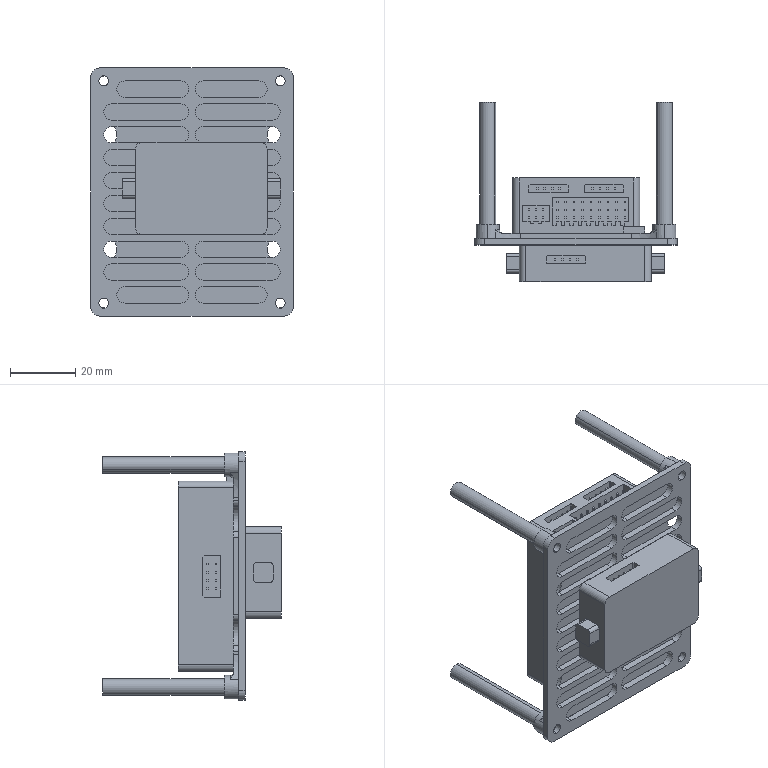Part | SolidWorks | 8 solids | 808 faces | box 62 x 54.7 x 76 mm | volume 57730 mm3 | plane 674 | cylinder 128 | torus 6 | commonest cylinder face diameters 5 x48 4 x16 2 x8 3 x8 3.1 x8 3.2 x8